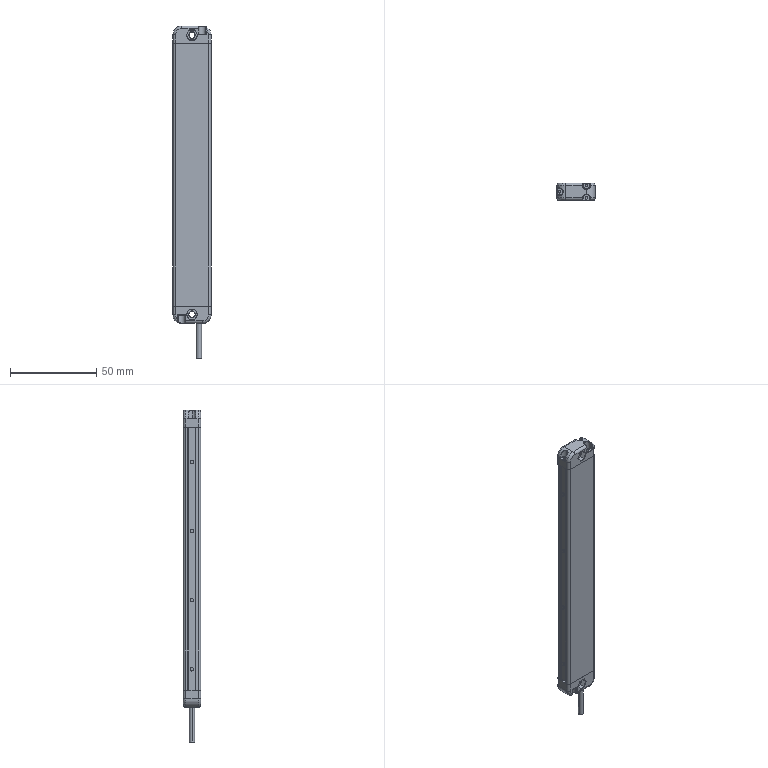Part | STEP file | Safety light curtain 4PLN-0440V1.201001 | 5 solids | 543 faces | box 22 x 10 x 192 mm | volume 17011 mm3 | cylinder 238 | plane 201 | torus 76 | spline 28 | commonest cylinder face diameters 0.4 x93 0.2 x26 3 x19 3.9 x16 0.6 x15 1.5 x12